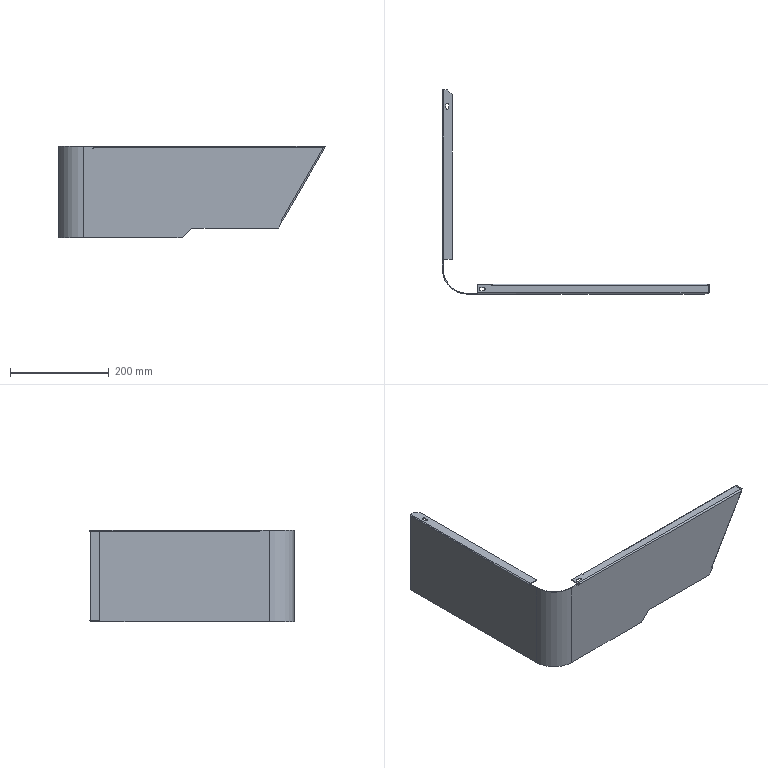Part | SolidWorks | features ICE 10, EdgeFlange 4, Chamfer 1, FlatPattern 1, Hem 1, SMBaseFlange 1, SheetMetal 1 | 1 solid | 98 faces | box 540.3 x 413 x 185.75 mm | volume 284651 mm3 | plane 72 | cylinder 22 | spline 4 | commonest cylinder face diameters 6 x4 6.4 x4 1 x3 4 x3 2 x2 5 x2